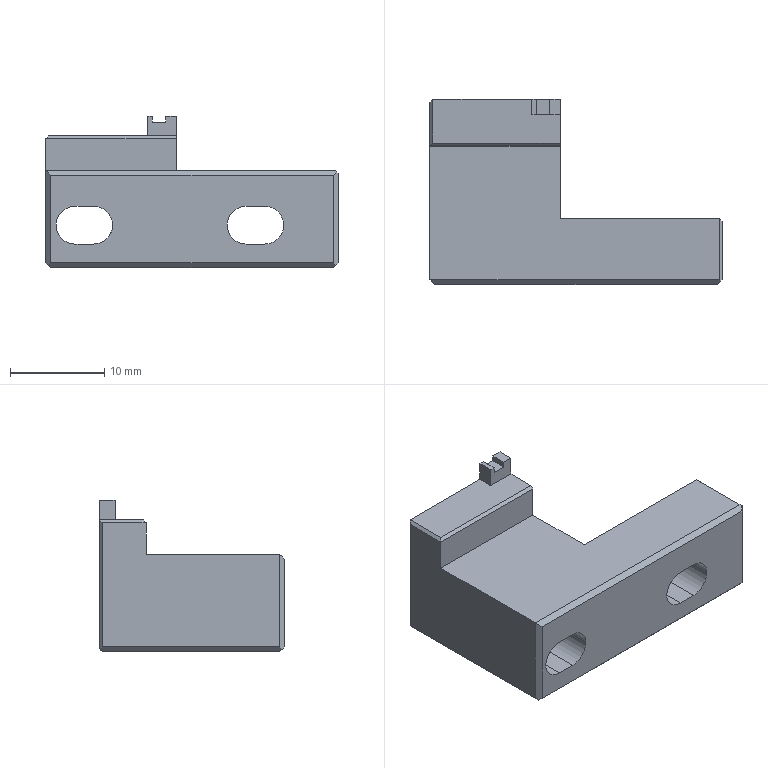Part | NX | 1 solid | 49 faces | box 31 x 19.62 x 16.052 mm | volume 3662 mm3 | plane 35 | cylinder 10 | cone 4 | commonest cylinder face diameters 4 x6 2.5 x2 3.3 x2